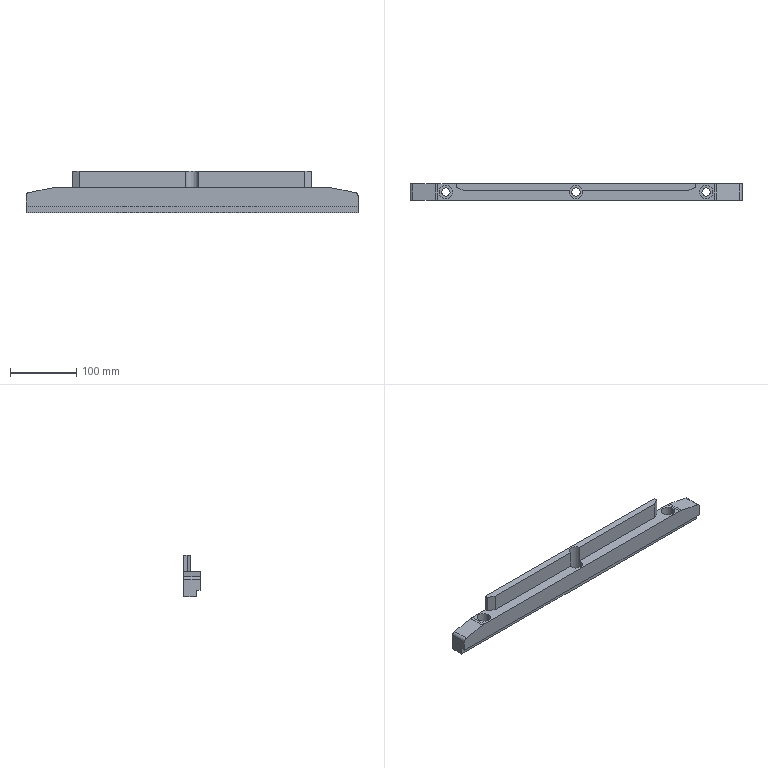NC program | NX | posted with a generic post | part box 500 x 25 x 62.5 mm
Lines 1 to 29 of 3905:
N10 G17 G21 G94 G90
(DRILLING_COPY_1 , TOOL : D6A45)
N12 T02 M6
N14 G54
N16 G17 G0 G90 X-196. Y0. S5000 M3
N18 G43 Z30. H2
N20 G94 G81 G98 Z-2.1 F250. R3.
N22 X0.
N24 X196.
N26 G80
N28 G0 X196. Y0. Z30.
N30 M5
(DRILLING_COPY_COPY_1 , TOOL : 12.5ZT)
N32 T12 M6
N34 G54
N36 G17 G0 G90 X0. Y0. S1200 M3
N38 G43 Z30. H12
N40 G94 G83 G98 Z-19.755 F250. Q2. R3.
N42 X-196.
N44 X196.
N46 G80
N48 G0 X196. Y0. Z30.
N50 M5